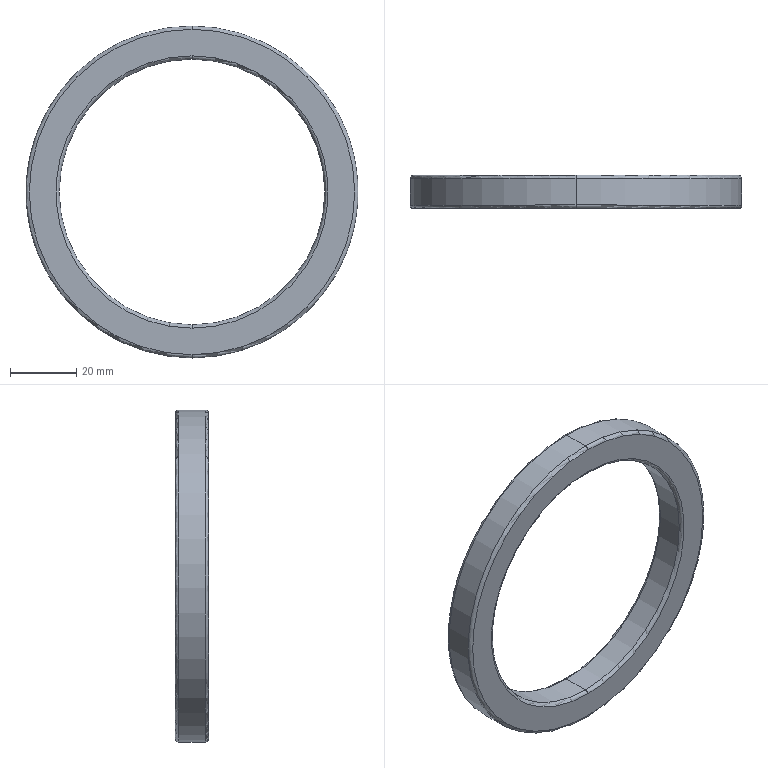Part | SolidWorks | features Extrusion 1, Fillet 1 | 1 solid | 14 faces | box 100 x 10 x 100 mm | volume 28032 mm3 | torus 8 | cylinder 4 | plane 2 | commonest cylinder face diameters 80 x2 100 x2
STEP:
#1=CARTESIAN_POINT('',(0.,10.,-41.));
#2=VERTEX_POINT('',#1);
#3=CARTESIAN_POINT('',(0.,10.,41.));
#4=VERTEX_POINT('',#3);
#5=CARTESIAN_POINT('',(0.,10.,0.));
#6=DIRECTION('',(0.,-1.,0.));
#7=DIRECTION('',(0.,0.,1.));
#8=AXIS2_PLACEMENT_3D('',#5,#6,#7);
#9=CIRCLE('',#8,41.);
#10=EDGE_CURVE('',#2,#4,#9,.T.);
#11=ORIENTED_EDGE('',*,*,#10,.F.);
#12=CARTESIAN_POINT('',(0.,9.,-40.));
#13=VERTEX_POINT('',#12);
#14=CARTESIAN_POINT('',(0.,9.,-41.));
#15=DIRECTION('',(1.,0.,0.));
#16=DIRECTION('',(0.,0.,-1.));
#17=AXIS2_PLACEMENT_3D('',#14,#15,#16);
#18=CIRCLE('',#17,1.);
#19=EDGE_CURVE('',#2,#13,#18,.T.);
#20=ORIENTED_EDGE('',*,*,#19,.T.);
#21=CARTESIAN_POINT('',(0.,9.,40.));
#22=VERTEX_POINT('',#21);
#23=CARTESIAN_POINT('',(0.,9.,0.));
#24=DIRECTION('',(0.,1.,0.));
#25=DIRECTION('',(0.,0.,1.));
#26=AXIS2_PLACEMENT_3D('',#23,#24,#25);
#27=CIRCLE('',#26,40.);
#28=EDGE_CURVE('',#22,#13,#27,.T.);
#29=ORIENTED_EDGE('',*,*,#28,.F.);
#30=CARTESIAN_POINT('',(0.,9.,41.));
#31=DIRECTION('',(-1.,0.,0.));
#32=DIRECTION('',(0.,0.,1.));
#33=AXIS2_PLACEMENT_3D('',#30,#31,#32);
#34=CIRCLE('',#33,1.);
#35=EDGE_CURVE('',#4,#22,#34,.T.);
#36=ORIENTED_EDGE('',*,*,#35,.F.);
#37=EDGE_LOOP('',(#11,#20,#29,#36));
#38=FACE_OUTER_BOUND('',#37,.T.);
#39=CARTESIAN_POINT('',(0.,9.,0.));
#40=DIRECTION('',(0.,1.,0.));
#41=DIRECTION('',(0.,0.,1.));
#42=AXIS2_PLACEMENT_3D('',#39,#40,#41);
#43=TOROIDAL_SURFACE('',#42,41.,1.);
#44=ADVANCED_FACE('',(#38),#43,.T.);
#45=CARTESIAN_POINT('',(0.,1.,-40.));
#46=VERTEX_POINT('',#45);
#47=CARTESIAN_POINT('',(0.,1.,40.));
#48=VERTEX_POINT('',#47);
#49=CARTESIAN_POINT('',(0.,1.,0.));
#50=DIRECTION('',(0.,-1.,0.));
#51=DIRECTION('',(0.,0.,1.));
#52=AXIS2_PLACEMENT_3D('',#49,#50,#51);
#53=CIRCLE('',#52,40.);
#54=EDGE_CURVE('',#46,#48,#53,.T.);
#55=ORIENTED_EDGE('',*,*,#54,.F.);
#56=CARTESIAN_POINT('',(0.,0.,-41.));
#57=VERTEX_POINT('',#56);
#58=CARTESIAN_POINT('',(0.,1.,-41.));
#59=DIRECTION('',(1.,0.,0.));
#60=DIRECTION('',(0.,0.,-1.));
#61=AXIS2_PLACEMENT_3D('',#58,#59,#60);
#62=CIRCLE('',#61,1.);
#63=EDGE_CURVE('',#46,#57,#62,.T.);
#64=ORIENTED_EDGE('',*,*,#63,.T.);
#65=CARTESIAN_POINT('',(0.,0.,41.));
#66=VERTEX_POINT('',#65);
#67=CARTESIAN_POINT('',(0.,0.,0.));
#68=DIRECTION('',(0.,1.,0.));
#69=DIRECTION('',(0.,0.,1.));
#70=AXIS2_PLACEMENT_3D('',#67,#68,#69);
#71=CIRCLE('',#70,41.);
#72=EDGE_CURVE('',#66,#57,#71,.T.);
#73=ORIENTED_EDGE('',*,*,#72,.F.);
#74=CARTESIAN_POINT('',(0.,1.,41.));
#75=DIRECTION('',(-1.,0.,0.));
#76=DIRECTION('',(0.,0.,1.));
#77=AXIS2_PLACEMENT_3D('',#74,#75,#76);
#78=CIRCLE('',#77,1.);
#79=EDGE_CURVE('',#48,#66,#78,.T.);
#80=ORIENTED_EDGE('',*,*,#79,.F.);
#81=EDGE_LOOP('',(#55,#64,#73,#80));
#82=FACE_OUTER_BOUND('',#81,.T.);
#83=CARTESIAN_POINT('',(0.,1.,0.));
#84=DIRECTION('',(0.,1.,0.));
#85=DIRECTION('',(0.,0.,1.));
#86=AXIS2_PLACEMENT_3D('',#83,#84,#85);
#87=TOROIDAL_SURFACE('',#86,41.,1.);
#88=ADVANCED_FACE('',(#82),#87,.T.);
#89=CARTESIAN_POINT('',(0.,9.,-50.));
#90=VERTEX_POINT('',#89);
#91=CARTESIAN_POINT('',(0.,9.,50.));
#92=VERTEX_POINT('',#91);
#93=CARTESIAN_POINT('',(0.,9.,0.));
#94=DIRECTION('',(0.,-1.,0.));
#95=DIRECTION('',(0.,0.,1.));
#96=AXIS2_PLACEMENT_3D('',#93,#94,#95);
#97=CIRCLE('',#96,50.);
#98=EDGE_CURVE('',#90,#92,#97,.T.);
#99=ORIENTED_EDGE('',*,*,#98,.F.);
#100=CARTESIAN_POINT('',(0.,10.,-49.));
#101=VERTEX_POINT('',#100);
#102=CARTESIAN_POINT('',(0.,9.,-49.));
#103=DIRECTION('',(1.,0.,0.));
#104=DIRECTION('',(0.,0.,-1.));
#105=AXIS2_PLACEMENT_3D('',#102,#103,#104);
#106=CIRCLE('',#105,1.);
#107=EDGE_CURVE('',#90,#101,#106,.T.);
#108=ORIENTED_EDGE('',*,*,#107,.T.);
#109=CARTESIAN_POINT('',(0.,10.,49.));
#110=VERTEX_POINT('',#109);
#111=CARTESIAN_POINT('',(0.,10.,0.));
#112=DIRECTION('',(0.,1.,0.));
#113=DIRECTION('',(0.,0.,1.));
#114=AXIS2_PLACEMENT_3D('',#111,#112,#113);
#115=CIRCLE('',#114,49.);
#116=EDGE_CURVE('',#110,#101,#115,.T.);
#117=ORIENTED_EDGE('',*,*,#116,.F.);
#118=CARTESIAN_POINT('',(0.,9.,49.));
#119=DIRECTION('',(-1.,0.,0.));
#120=DIRECTION('',(0.,0.,1.));
#121=AXIS2_PLACEMENT_3D('',#118,#119,#120);
#122=CIRCLE('',#121,1.);
#123=EDGE_CURVE('',#92,#110,#122,.T.);
#124=ORIENTED_EDGE('',*,*,#123,.F.);
#125=EDGE_LOOP('',(#99,#108,#117,#124));
#126=FACE_OUTER_BOUND('',#125,.T.);
#127=CARTESIAN_POINT('',(0.,9.,0.));
#128=DIRECTION('',(0.,1.,0.));
#129=DIRECTION('',(0.,0.,1.));
#130=AXIS2_PLACEMENT_3D('',#127,#128,#129);
#131=TOROIDAL_SURFACE('',#130,49.,1.);
#132=ADVANCED_FACE('',(#126),#131,.T.);
#133=CARTESIAN_POINT('',(0.,0.,-49.));
#134=VERTEX_POINT('',#133);
#135=CARTESIAN_POINT('',(0.,0.,49.));
#136=VERTEX_POINT('',#135);
#137=CARTESIAN_POINT('',(0.,0.,0.));
#138=DIRECTION('',(0.,-1.,0.));
#139=DIRECTION('',(0.,0.,1.));
#140=AXIS2_PLACEMENT_3D('',#137,#138,#139);
#141=CIRCLE('',#140,49.);
#142=EDGE_CURVE('',#134,#136,#141,.T.);
#143=ORIENTED_EDGE('',*,*,#142,.F.);
#144=CARTESIAN_POINT('',(0.,1.,-50.));
#145=VERTEX_POINT('',#144);
#146=CARTESIAN_POINT('',(0.,1.,-49.));
#147=DIRECTION('',(1.,0.,0.));
#148=DIRECTION('',(0.,0.,-1.));
#149=AXIS2_PLACEMENT_3D('',#146,#147,#148);
#150=CIRCLE('',#149,1.);
#151=EDGE_CURVE('',#134,#145,#150,.T.);
#152=ORIENTED_EDGE('',*,*,#151,.T.);
#153=CARTESIAN_POINT('',(0.,1.,50.));
#154=VERTEX_POINT('',#153);
#155=CARTESIAN_POINT('',(0.,1.,0.));
#156=DIRECTION('',(0.,1.,0.));
#157=DIRECTION('',(0.,0.,1.));
#158=AXIS2_PLACEMENT_3D('',#155,#156,#157);
#159=CIRCLE('',#158,50.);
#160=EDGE_CURVE('',#154,#145,#159,.T.);
#161=ORIENTED_EDGE('',*,*,#160,.F.);
#162=CARTESIAN_POINT('',(0.,1.,49.));
#163=DIRECTION('',(-1.,0.,0.));
#164=DIRECTION('',(0.,0.,1.));
#165=AXIS2_PLACEMENT_3D('',#162,#163,#164);
#166=CIRCLE('',#165,1.);
#167=EDGE_CURVE('',#136,#154,#166,.T.);
#168=ORIENTED_EDGE('',*,*,#167,.F.);
#169=EDGE_LOOP('',(#143,#152,#161,#168));
#170=FACE_OUTER_BOUND('',#169,.T.);
#171=CARTESIAN_POINT('',(0.,1.,0.));
#172=DIRECTION('',(0.,1.,0.));
#173=DIRECTION('',(0.,0.,1.));
#174=AXIS2_PLACEMENT_3D('',#171,#172,#173);
#175=TOROIDAL_SURFACE('',#174,49.,1.);
#176=ADVANCED_FACE('',(#170),#175,.T.);
#177=CARTESIAN_POINT('',(0.,9.,0.));
#178=DIRECTION('',(0.,1.,0.));
#179=DIRECTION('',(0.,0.,1.));
#180=AXIS2_PLACEMENT_3D('',#177,#178,#179);
#181=CIRCLE('',#180,40.);
#182=EDGE_CURVE('',#13,#22,#181,.T.);
#183=ORIENTED_EDGE('',*,*,#182,.T.);
#184=CARTESIAN_POINT('',(0.,10.,40.));
#185=DIRECTION('',(0.,-1.,0.));
#186=VECTOR('',#185,1000.);
#187=LINE('',#184,#186);
#188=EDGE_CURVE('',#22,#48,#187,.T.);
#189=ORIENTED_EDGE('',*,*,#188,.T.);
#190=CARTESIAN_POINT('',(0.,1.,0.));
#191=DIRECTION('',(0.,-1.,0.));
#192=DIRECTION('',(0.,0.,1.));
#193=AXIS2_PLACEMENT_3D('',#190,#191,#192);
#194=CIRCLE('',#193,40.);
#195=EDGE_CURVE('',#48,#46,#194,.T.);
#196=ORIENTED_EDGE('',*,*,#195,.T.);
#197=CARTESIAN_POINT('',(0.,10.,-40.));
#198=DIRECTION('',(0.,-1.,0.));
#199=VECTOR('',#198,1000.);
#200=LINE('',#197,#199);
#201=EDGE_CURVE('',#13,#46,#200,.T.);
#202=ORIENTED_EDGE('',*,*,#201,.F.);
#203=EDGE_LOOP('',(#183,#189,#196,#202));
#204=FACE_OUTER_BOUND('',#203,.T.);
#205=CARTESIAN_POINT('',(0.,10.,0.));
#206=DIRECTION('',(0.,-1.,0.));
#207=DIRECTION('',(0.,0.,-1.));
#208=AXIS2_PLACEMENT_3D('',#205,#206,#207);
#209=CYLINDRICAL_SURFACE('',#208,40.);
#210=ADVANCED_FACE('',(#204),#209,.F.);
#211=ORIENTED_EDGE('',*,*,#98,.T.);
#212=CARTESIAN_POINT('',(0.,10.,50.));
#213=DIRECTION('',(0.,-1.,0.));
#214=VECTOR('',#213,1000.);
#215=LINE('',#212,#214);
#216=EDGE_CURVE('',#92,#154,#215,.T.);
#217=ORIENTED_EDGE('',*,*,#216,.T.);
#218=ORIENTED_EDGE('',*,*,#160,.T.);
#219=CARTESIAN_POINT('',(0.,10.,-50.));
#220=DIRECTION('',(0.,-1.,0.));
#221=VECTOR('',#220,1000.);
#222=LINE('',#219,#221);
#223=EDGE_CURVE('',#90,#145,#222,.T.);
#224=ORIENTED_EDGE('',*,*,#223,.F.);
#225=EDGE_LOOP('',(#211,#217,#218,#224));
#226=FACE_OUTER_BOUND('',#225,.T.);
#227=CARTESIAN_POINT('',(0.,10.,0.));
#228=DIRECTION('',(0.,-1.,0.));
#229=DIRECTION('',(0.,0.,-1.));
#230=AXIS2_PLACEMENT_3D('',#227,#228,#229);
#231=CYLINDRICAL_SURFACE('',#230,50.);
#232=ADVANCED_FACE('',(#226),#231,.T.);
#233=ORIENTED_EDGE('',*,*,#116,.T.);
#234=CARTESIAN_POINT('',(0.,10.,0.));
#235=DIRECTION('',(0.,1.,0.));
#236=DIRECTION('',(0.,0.,1.));
#237=AXIS2_PLACEMENT_3D('',#234,#235,#236);
#238=CIRCLE('',#237,49.);
#239=EDGE_CURVE('',#101,#110,#238,.T.);
#240=ORIENTED_EDGE('',*,*,#239,.T.);
#241=EDGE_LOOP('',(#233,#240));
#242=FACE_OUTER_BOUND('',#241,.T.);
#243=CARTESIAN_POINT('',(0.,10.,0.));
#244=DIRECTION('',(0.,-1.,0.));
#245=DIRECTION('',(0.,0.,1.));
#246=AXIS2_PLACEMENT_3D('',#243,#244,#245);
#247=CIRCLE('',#246,41.);
#248=EDGE_CURVE('',#4,#2,#247,.T.);
#249=ORIENTED_EDGE('',*,*,#248,.T.);
#250=ORIENTED_EDGE('',*,*,#10,.T.);
#251=EDGE_LOOP('',(#249,#250));
#252=FACE_BOUND('',#251,.T.);
#253=CARTESIAN_POINT('',(0.,10.,0.));
#254=DIRECTION('',(0.,1.,0.));
#255=DIRECTION('',(0.,0.,1.));
#256=AXIS2_PLACEMENT_3D('',#253,#254,#255);
#257=PLANE('',#256);
#258=ADVANCED_FACE('',(#242,#252),#257,.T.);
#259=CARTESIAN_POINT('',(0.,0.,0.));
#260=DIRECTION('',(0.,-1.,0.));
#261=DIRECTION('',(0.,0.,1.));
#262=AXIS2_PLACEMENT_3D('',#259,#260,#261);
#263=CIRCLE('',#262,49.);
#264=EDGE_CURVE('',#136,#134,#263,.T.);
#265=ORIENTED_EDGE('',*,*,#264,.T.);
#266=ORIENTED_EDGE('',*,*,#142,.T.);
#267=EDGE_LOOP('',(#265,#266));
#268=FACE_OUTER_BOUND('',#267,.T.);
#269=ORIENTED_EDGE('',*,*,#72,.T.);
#270=CARTESIAN_POINT('',(0.,0.,0.));
#271=DIRECTION('',(0.,1.,0.));
#272=DIRECTION('',(0.,0.,1.));
#273=AXIS2_PLACEMENT_3D('',#270,#271,#272);
#274=CIRCLE('',#273,41.);
#275=EDGE_CURVE('',#57,#66,#274,.T.);
#276=ORIENTED_EDGE('',*,*,#275,.T.);
#277=EDGE_LOOP('',(#269,#276));
#278=FACE_BOUND('',#277,.T.);
#279=CARTESIAN_POINT('',(0.,0.,0.));
#280=DIRECTION('',(0.,1.,0.));
#281=DIRECTION('',(0.,0.,1.));
#282=AXIS2_PLACEMENT_3D('',#279,#280,#281);
#283=PLANE('',#282);
#284=ADVANCED_FACE('',(#268,#278),#283,.F.);
#285=ORIENTED_EDGE('',*,*,#216,.F.);
#286=CARTESIAN_POINT('',(0.,9.,0.));
#287=DIRECTION('',(0.,-1.,0.));
#288=DIRECTION('',(0.,0.,1.));
#289=AXIS2_PLACEMENT_3D('',#286,#287,#288);
#290=CIRCLE('',#289,50.);
#291=EDGE_CURVE('',#92,#90,#290,.T.);
#292=ORIENTED_EDGE('',*,*,#291,.T.);
#293=ORIENTED_EDGE('',*,*,#223,.T.);
#294=CARTESIAN_POINT('',(0.,1.,0.));
#295=DIRECTION('',(0.,1.,0.));
#296=DIRECTION('',(0.,0.,1.));
#297=AXIS2_PLACEMENT_3D('',#294,#295,#296);
#298=CIRCLE('',#297,50.);
#299=EDGE_CURVE('',#145,#154,#298,.T.);
#300=ORIENTED_EDGE('',*,*,#299,.T.);
#301=EDGE_LOOP('',(#285,#292,#293,#300));
#302=FACE_OUTER_BOUND('',#301,.T.);
#303=CARTESIAN_POINT('',(0.,10.,0.));
#304=DIRECTION('',(0.,-1.,0.));
#305=DIRECTION('',(0.,0.,-1.));
#306=AXIS2_PLACEMENT_3D('',#303,#304,#305);
#307=CYLINDRICAL_SURFACE('',#306,50.);
#308=ADVANCED_FACE('',(#302),#307,.T.);
#309=ORIENTED_EDGE('',*,*,#188,.F.);
#310=ORIENTED_EDGE('',*,*,#28,.T.);
#311=ORIENTED_EDGE('',*,*,#201,.T.);
#312=ORIENTED_EDGE('',*,*,#54,.T.);
#313=EDGE_LOOP('',(#309,#310,#311,#312));
#314=FACE_OUTER_BOUND('',#313,.T.);
#315=CARTESIAN_POINT('',(0.,10.,0.));
#316=DIRECTION('',(0.,-1.,0.));
#317=DIRECTION('',(0.,0.,-1.));
#318=AXIS2_PLACEMENT_3D('',#315,#316,#317);
#319=CYLINDRICAL_SURFACE('',#318,40.);
#320=ADVANCED_FACE('',(#314),#319,.F.);
#321=ORIENTED_EDGE('',*,*,#151,.F.);
#322=ORIENTED_EDGE('',*,*,#264,.F.);
#323=ORIENTED_EDGE('',*,*,#167,.T.);
#324=ORIENTED_EDGE('',*,*,#299,.F.);
#325=EDGE_LOOP('',(#321,#322,#323,#324));
#326=FACE_OUTER_BOUND('',#325,.T.);
#327=CARTESIAN_POINT('',(0.,1.,0.));
#328=DIRECTION('',(0.,1.,0.));
#329=DIRECTION('',(0.,0.,1.));
#330=AXIS2_PLACEMENT_3D('',#327,#328,#329);
#331=TOROIDAL_SURFACE('',#330,49.,1.);
#332=ADVANCED_FACE('',(#326),#331,.T.);
#333=ORIENTED_EDGE('',*,*,#107,.F.);
#334=ORIENTED_EDGE('',*,*,#291,.F.);
#335=ORIENTED_EDGE('',*,*,#123,.T.);
#336=ORIENTED_EDGE('',*,*,#239,.F.);
#337=EDGE_LOOP('',(#333,#334,#335,#336));
#338=FACE_OUTER_BOUND('',#337,.T.);
#339=CARTESIAN_POINT('',(0.,9.,0.));
#340=DIRECTION('',(0.,1.,0.));
#341=DIRECTION('',(0.,0.,1.));
#342=AXIS2_PLACEMENT_3D('',#339,#340,#341);
#343=TOROIDAL_SURFACE('',#342,49.,1.);
#344=ADVANCED_FACE('',(#338),#343,.T.);
#345=ORIENTED_EDGE('',*,*,#63,.F.);
#346=ORIENTED_EDGE('',*,*,#195,.F.);
#347=ORIENTED_EDGE('',*,*,#79,.T.);
#348=ORIENTED_EDGE('',*,*,#275,.F.);
#349=EDGE_LOOP('',(#345,#346,#347,#348));
#350=FACE_OUTER_BOUND('',#349,.T.);
#351=CARTESIAN_POINT('',(0.,1.,0.));
#352=DIRECTION('',(0.,1.,0.));
#353=DIRECTION('',(0.,0.,1.));
#354=AXIS2_PLACEMENT_3D('',#351,#352,#353);
#355=TOROIDAL_SURFACE('',#354,41.,1.);
#356=ADVANCED_FACE('',(#350),#355,.T.);
#357=ORIENTED_EDGE('',*,*,#19,.F.);
#358=ORIENTED_EDGE('',*,*,#248,.F.);
#359=ORIENTED_EDGE('',*,*,#35,.T.);
#360=ORIENTED_EDGE('',*,*,#182,.F.);
#361=EDGE_LOOP('',(#357,#358,#359,#360));
#362=FACE_OUTER_BOUND('',#361,.T.);
#363=CARTESIAN_POINT('',(0.,9.,0.));
#364=DIRECTION('',(0.,1.,0.));
#365=DIRECTION('',(0.,0.,1.));
#366=AXIS2_PLACEMENT_3D('',#363,#364,#365);
#367=TOROIDAL_SURFACE('',#366,41.,1.);
#368=ADVANCED_FACE('',(#362),#367,.T.);
#369=CLOSED_SHELL('',(#44,#88,#132,#176,#210,#232,#258,#284,#308,#320,#332,#344,#356,#368));
#370=MANIFOLD_SOLID_BREP('',#369);
#371=CARTESIAN_POINT('',(0.,0.,0.));
#372=DIRECTION('',(0.,0.,1.));
#373=DIRECTION('',(1.,0.,0.));
#374=AXIS2_PLACEMENT_3D('',#371,#372,#373);
#375=(LENGTH_UNIT()NAMED_UNIT(*)SI_UNIT(.MILLI.,.METRE.));
#376=UNCERTAINTY_MEASURE_WITH_UNIT(LENGTH_MEASURE(0.00001),#375,'','');
#377=(NAMED_UNIT(*)PLANE_ANGLE_UNIT()SI_UNIT($,.RADIAN.));
#378=(NAMED_UNIT(*)SI_UNIT($,.STERADIAN.)SOLID_ANGLE_UNIT());
#379=(GEOMETRIC_REPRESENTATION_CONTEXT(3)GLOBAL_UNCERTAINTY_ASSIGNED_CONTEXT((#376))GLOBAL_UNIT_ASSIGNED_CONTEXT((#375,#377,#378))REPRESENTATION_CONTEXT('',''));
#380=ADVANCED_BREP_SHAPE_REPRESENTATION('',(#370,#374),#379);